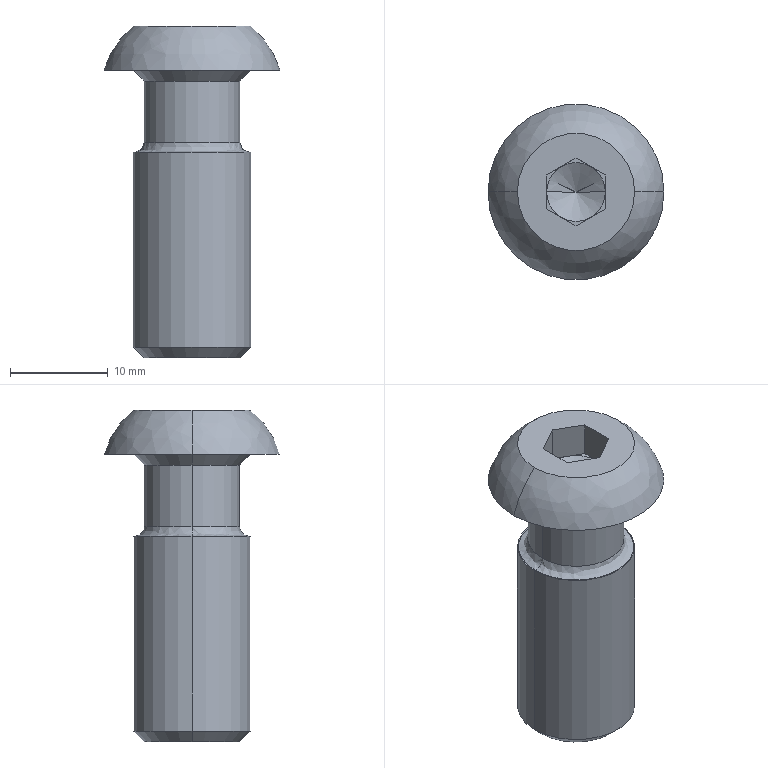Part | STEP file | 0245_Z_016_HCJ8_2 | 1 solid | 30 faces | box 18 x 18 x 33.9 mm | volume 3765 mm3 | plane 16 | cone 6 | spline 4 | cylinder 4 | commonest cylinder face diameters 9.8 x2 12 x2